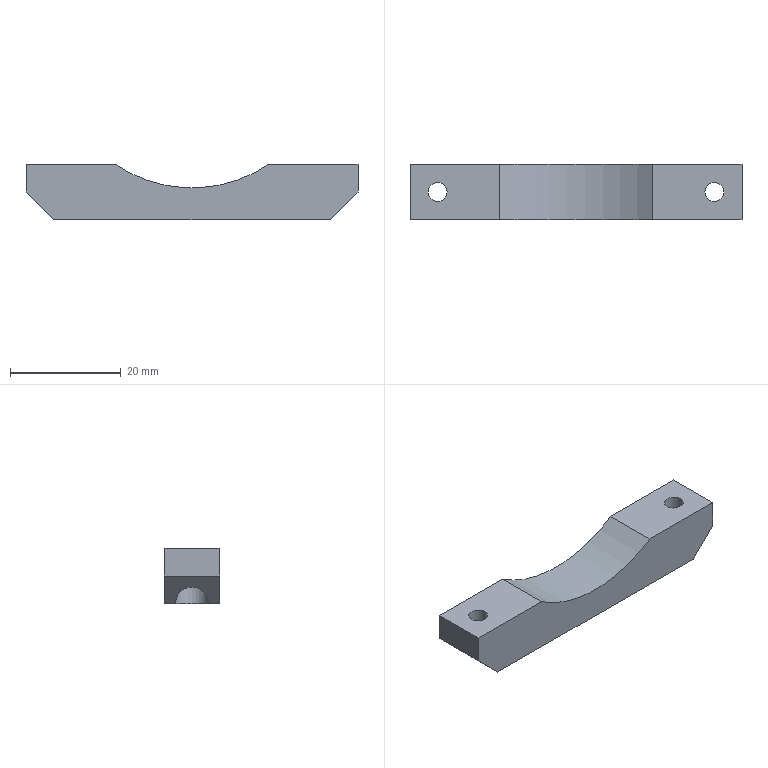Part | STEP file | SynoNew-0304-067 | 1 solid | 16 faces | box 60 x 10 x 10 mm | volume 4574 mm3 | plane 11 | cylinder 5 | commonest cylinder face diameters 3.4 x2 6 x2 49.5 x1
STEP:
#1=CARTESIAN_POINT('',(0.,10.,-5.));
#2=VERTEX_POINT('',#1);
#3=CARTESIAN_POINT('',(0.,10.,0.));
#4=VERTEX_POINT('',#3);
#5=CARTESIAN_POINT('',(0.,10.,-5.));
#6=DIRECTION('',(0.,0.,1.));
#7=VECTOR('',#6,5.);
#8=LINE('',#5,#7);
#9=EDGE_CURVE('',#2,#4,#8,.T.);
#10=ORIENTED_EDGE('',*,*,#9,.F.);
#11=CARTESIAN_POINT('',(0.,0.,-5.));
#12=VERTEX_POINT('',#11);
#13=CARTESIAN_POINT('',(0.,10.,-5.));
#14=DIRECTION('',(0.,-1.,0.));
#15=VECTOR('',#14,10.);
#16=LINE('',#13,#15);
#17=EDGE_CURVE('',#2,#12,#16,.T.);
#18=ORIENTED_EDGE('',*,*,#17,.T.);
#19=CARTESIAN_POINT('',(0.,0.,0.));
#20=VERTEX_POINT('',#19);
#21=CARTESIAN_POINT('',(0.,0.,-5.));
#22=DIRECTION('',(0.,0.,1.));
#23=VECTOR('',#22,5.);
#24=LINE('',#21,#23);
#25=EDGE_CURVE('',#12,#20,#24,.T.);
#26=ORIENTED_EDGE('',*,*,#25,.T.);
#27=CARTESIAN_POINT('',(0.,10.,0.));
#28=DIRECTION('',(0.,-1.,0.));
#29=VECTOR('',#28,10.);
#30=LINE('',#27,#29);
#31=EDGE_CURVE('',#4,#20,#30,.T.);
#32=ORIENTED_EDGE('',*,*,#31,.F.);
#33=EDGE_LOOP('',(#10,#18,#26,#32));
#34=FACE_OUTER_BOUND('',#33,.T.);
#35=CARTESIAN_POINT('',(0.,10.,0.));
#36=DIRECTION('',(1.,0.,0.));
#37=DIRECTION('',(0.,0.,-1.));
#38=AXIS2_PLACEMENT_3D('',#35,#36,#37);
#39=PLANE('',#38);
#40=ADVANCED_FACE('',(#34),#39,.F.);
#41=CARTESIAN_POINT('',(16.132,0.,0.));
#42=VERTEX_POINT('',#41);
#43=CARTESIAN_POINT('',(0.,0.,0.));
#44=DIRECTION('',(1.,0.,0.));
#45=VECTOR('',#44,16.132);
#46=LINE('',#43,#45);
#47=EDGE_CURVE('',#20,#42,#46,.T.);
#48=ORIENTED_EDGE('',*,*,#47,.T.);
#49=CARTESIAN_POINT('',(16.132,10.,0.));
#50=VERTEX_POINT('',#49);
#51=CARTESIAN_POINT('',(16.132,10.,0.));
#52=DIRECTION('',(0.,-1.,0.));
#53=VECTOR('',#52,10.);
#54=LINE('',#51,#53);
#55=EDGE_CURVE('',#50,#42,#54,.T.);
#56=ORIENTED_EDGE('',*,*,#55,.F.);
#57=CARTESIAN_POINT('',(0.,10.,0.));
#58=DIRECTION('',(1.,0.,0.));
#59=VECTOR('',#58,16.132);
#60=LINE('',#57,#59);
#61=EDGE_CURVE('',#4,#50,#60,.T.);
#62=ORIENTED_EDGE('',*,*,#61,.F.);
#63=ORIENTED_EDGE('',*,*,#31,.T.);
#64=EDGE_LOOP('',(#48,#56,#62,#63));
#65=FACE_OUTER_BOUND('',#64,.T.);
#66=CARTESIAN_POINT('',(3.3,5.,0.));
#67=VERTEX_POINT('',#66);
#68=CARTESIAN_POINT('',(6.7,5.,0.));
#69=VERTEX_POINT('',#68);
#70=CARTESIAN_POINT('',(5.,5.,0.));
#71=DIRECTION('',(0.,0.,-1.));
#72=DIRECTION('',(-1.,0.,0.));
#73=AXIS2_PLACEMENT_3D('',#70,#71,#72);
#74=CIRCLE('',#73,1.7);
#75=EDGE_CURVE('',#67,#69,#74,.T.);
#76=ORIENTED_EDGE('',*,*,#75,.T.);
#77=CARTESIAN_POINT('',(5.,5.,0.));
#78=DIRECTION('',(0.,0.,-1.));
#79=DIRECTION('',(-1.,0.,0.));
#80=AXIS2_PLACEMENT_3D('',#77,#78,#79);
#81=CIRCLE('',#80,1.7);
#82=EDGE_CURVE('',#69,#67,#81,.T.);
#83=ORIENTED_EDGE('',*,*,#82,.T.);
#84=EDGE_LOOP('',(#76,#83));
#85=FACE_BOUND('',#84,.T.);
#86=CARTESIAN_POINT('',(0.,10.,0.));
#87=DIRECTION('',(0.,0.,-1.));
#88=DIRECTION('',(-1.,0.,0.));
#89=AXIS2_PLACEMENT_3D('',#86,#87,#88);
#90=PLANE('',#89);
#91=ADVANCED_FACE('',(#65,#85),#90,.F.);
#92=CARTESIAN_POINT('',(43.868,0.,0.));
#93=VERTEX_POINT('',#92);
#94=CARTESIAN_POINT('',(30.,0.,20.5));
#95=DIRECTION('',(0.,-1.,0.));
#96=DIRECTION('',(0.,0.,1.));
#97=AXIS2_PLACEMENT_3D('',#94,#95,#96);
#98=CIRCLE('',#97,24.75);
#99=EDGE_CURVE('',#42,#93,#98,.T.);
#100=ORIENTED_EDGE('',*,*,#99,.T.);
#101=CARTESIAN_POINT('',(43.868,10.,0.));
#102=VERTEX_POINT('',#101);
#103=CARTESIAN_POINT('',(43.868,10.,0.));
#104=DIRECTION('',(0.,-1.,0.));
#105=VECTOR('',#104,10.);
#106=LINE('',#103,#105);
#107=EDGE_CURVE('',#102,#93,#106,.T.);
#108=ORIENTED_EDGE('',*,*,#107,.F.);
#109=CARTESIAN_POINT('',(30.,10.,20.5));
#110=DIRECTION('',(0.,-1.,0.));
#111=DIRECTION('',(0.,0.,1.));
#112=AXIS2_PLACEMENT_3D('',#109,#110,#111);
#113=CIRCLE('',#112,24.75);
#114=EDGE_CURVE('',#50,#102,#113,.T.);
#115=ORIENTED_EDGE('',*,*,#114,.F.);
#116=ORIENTED_EDGE('',*,*,#55,.T.);
#117=EDGE_LOOP('',(#100,#108,#115,#116));
#118=FACE_OUTER_BOUND('',#117,.T.);
#119=CARTESIAN_POINT('',(30.,10.,20.5));
#120=DIRECTION('',(0.,-1.,0.));
#121=DIRECTION('',(0.,0.,-1.));
#122=AXIS2_PLACEMENT_3D('',#119,#120,#121);
#123=CYLINDRICAL_SURFACE('',#122,24.75);
#124=ADVANCED_FACE('',(#118),#123,.F.);
#125=CARTESIAN_POINT('',(60.,0.,0.));
#126=VERTEX_POINT('',#125);
#127=CARTESIAN_POINT('',(43.868,0.,0.));
#128=DIRECTION('',(1.,0.,0.));
#129=VECTOR('',#128,16.132);
#130=LINE('',#127,#129);
#131=EDGE_CURVE('',#93,#126,#130,.T.);
#132=ORIENTED_EDGE('',*,*,#131,.T.);
#133=CARTESIAN_POINT('',(60.,10.,0.));
#134=VERTEX_POINT('',#133);
#135=CARTESIAN_POINT('',(60.,10.,0.));
#136=DIRECTION('',(0.,-1.,0.));
#137=VECTOR('',#136,10.);
#138=LINE('',#135,#137);
#139=EDGE_CURVE('',#134,#126,#138,.T.);
#140=ORIENTED_EDGE('',*,*,#139,.F.);
#141=CARTESIAN_POINT('',(43.868,10.,0.));
#142=DIRECTION('',(1.,0.,0.));
#143=VECTOR('',#142,16.132);
#144=LINE('',#141,#143);
#145=EDGE_CURVE('',#102,#134,#144,.T.);
#146=ORIENTED_EDGE('',*,*,#145,.F.);
#147=ORIENTED_EDGE('',*,*,#107,.T.);
#148=EDGE_LOOP('',(#132,#140,#146,#147));
#149=FACE_OUTER_BOUND('',#148,.T.);
#150=CARTESIAN_POINT('',(53.3,5.,0.));
#151=VERTEX_POINT('',#150);
#152=CARTESIAN_POINT('',(56.7,5.,0.));
#153=VERTEX_POINT('',#152);
#154=CARTESIAN_POINT('',(55.,5.,0.));
#155=DIRECTION('',(0.,0.,-1.));
#156=DIRECTION('',(-1.,0.,0.));
#157=AXIS2_PLACEMENT_3D('',#154,#155,#156);
#158=CIRCLE('',#157,1.7);
#159=EDGE_CURVE('',#151,#153,#158,.T.);
#160=ORIENTED_EDGE('',*,*,#159,.T.);
#161=CARTESIAN_POINT('',(55.,5.,0.));
#162=DIRECTION('',(0.,0.,-1.));
#163=DIRECTION('',(-1.,0.,0.));
#164=AXIS2_PLACEMENT_3D('',#161,#162,#163);
#165=CIRCLE('',#164,1.7);
#166=EDGE_CURVE('',#153,#151,#165,.T.);
#167=ORIENTED_EDGE('',*,*,#166,.T.);
#168=EDGE_LOOP('',(#160,#167));
#169=FACE_BOUND('',#168,.T.);
#170=CARTESIAN_POINT('',(43.868,10.,0.));
#171=DIRECTION('',(0.,0.,-1.));
#172=DIRECTION('',(-1.,0.,0.));
#173=AXIS2_PLACEMENT_3D('',#170,#171,#172);
#174=PLANE('',#173);
#175=ADVANCED_FACE('',(#149,#169),#174,.F.);
#176=CARTESIAN_POINT('',(60.,0.,-5.));
#177=VERTEX_POINT('',#176);
#178=CARTESIAN_POINT('',(60.,0.,0.));
#179=DIRECTION('',(0.,0.,-1.));
#180=VECTOR('',#179,5.);
#181=LINE('',#178,#180);
#182=EDGE_CURVE('',#126,#177,#181,.T.);
#183=ORIENTED_EDGE('',*,*,#182,.T.);
#184=CARTESIAN_POINT('',(60.,10.,-5.));
#185=VERTEX_POINT('',#184);
#186=CARTESIAN_POINT('',(60.,0.,-5.));
#187=DIRECTION('',(0.,1.,0.));
#188=VECTOR('',#187,10.);
#189=LINE('',#186,#188);
#190=EDGE_CURVE('',#177,#185,#189,.T.);
#191=ORIENTED_EDGE('',*,*,#190,.T.);
#192=CARTESIAN_POINT('',(60.,10.,0.));
#193=DIRECTION('',(0.,0.,-1.));
#194=VECTOR('',#193,5.);
#195=LINE('',#192,#194);
#196=EDGE_CURVE('',#134,#185,#195,.T.);
#197=ORIENTED_EDGE('',*,*,#196,.F.);
#198=ORIENTED_EDGE('',*,*,#139,.T.);
#199=EDGE_LOOP('',(#183,#191,#197,#198));
#200=FACE_OUTER_BOUND('',#199,.T.);
#201=CARTESIAN_POINT('',(60.,10.,0.));
#202=DIRECTION('',(-1.,0.,0.));
#203=DIRECTION('',(0.,0.,1.));
#204=AXIS2_PLACEMENT_3D('',#201,#202,#203);
#205=PLANE('',#204);
#206=ADVANCED_FACE('',(#200),#205,.F.);
#207=CARTESIAN_POINT('',(55.,10.,-10.));
#208=VERTEX_POINT('',#207);
#209=CARTESIAN_POINT('',(55.,8.,-10.));
#210=VERTEX_POINT('',#209);
#211=CARTESIAN_POINT('',(55.,10.,-10.));
#212=DIRECTION('',(0.,-1.,0.));
#213=VECTOR('',#212,2.);
#214=LINE('',#211,#213);
#215=EDGE_CURVE('',#208,#210,#214,.T.);
#216=ORIENTED_EDGE('',*,*,#215,.T.);
#217=CARTESIAN_POINT('',(55.,2.,-10.));
#218=VERTEX_POINT('',#217);
#219=CARTESIAN_POINT('',(55.,5.,-10.));
#220=DIRECTION('',(0.,0.,-1.));
#221=DIRECTION('',(-1.,0.,0.));
#222=AXIS2_PLACEMENT_3D('',#219,#220,#221);
#223=CIRCLE('',#222,3.);
#224=EDGE_CURVE('',#218,#210,#223,.T.);
#225=ORIENTED_EDGE('',*,*,#224,.F.);
#226=CARTESIAN_POINT('',(55.,0.,-10.));
#227=VERTEX_POINT('',#226);
#228=CARTESIAN_POINT('',(55.,2.,-10.));
#229=DIRECTION('',(0.,-1.,0.));
#230=VECTOR('',#229,2.);
#231=LINE('',#228,#230);
#232=EDGE_CURVE('',#218,#227,#231,.T.);
#233=ORIENTED_EDGE('',*,*,#232,.T.);
#234=CARTESIAN_POINT('',(5.,0.,-10.));
#235=VERTEX_POINT('',#234);
#236=CARTESIAN_POINT('',(55.,0.,-10.));
#237=DIRECTION('',(-1.,0.,0.));
#238=VECTOR('',#237,50.);
#239=LINE('',#236,#238);
#240=EDGE_CURVE('',#227,#235,#239,.T.);
#241=ORIENTED_EDGE('',*,*,#240,.T.);
#242=CARTESIAN_POINT('',(5.,2.,-10.));
#243=VERTEX_POINT('',#242);
#244=CARTESIAN_POINT('',(5.,0.,-10.));
#245=DIRECTION('',(0.,1.,0.));
#246=VECTOR('',#245,2.);
#247=LINE('',#244,#246);
#248=EDGE_CURVE('',#235,#243,#247,.T.);
#249=ORIENTED_EDGE('',*,*,#248,.T.);
#250=CARTESIAN_POINT('',(8.,5.,-10.));
#251=VERTEX_POINT('',#250);
#252=CARTESIAN_POINT('',(5.,5.,-10.));
#253=DIRECTION('',(0.,0.,-1.));
#254=DIRECTION('',(-1.,0.,0.));
#255=AXIS2_PLACEMENT_3D('',#252,#253,#254);
#256=CIRCLE('',#255,3.);
#257=EDGE_CURVE('',#251,#243,#256,.T.);
#258=ORIENTED_EDGE('',*,*,#257,.F.);
#259=CARTESIAN_POINT('',(5.,8.,-10.));
#260=VERTEX_POINT('',#259);
#261=CARTESIAN_POINT('',(5.,5.,-10.));
#262=DIRECTION('',(0.,0.,-1.));
#263=DIRECTION('',(-1.,0.,0.));
#264=AXIS2_PLACEMENT_3D('',#261,#262,#263);
#265=CIRCLE('',#264,3.);
#266=EDGE_CURVE('',#260,#251,#265,.T.);
#267=ORIENTED_EDGE('',*,*,#266,.F.);
#268=CARTESIAN_POINT('',(5.,10.,-10.));
#269=VERTEX_POINT('',#268);
#270=CARTESIAN_POINT('',(5.,8.,-10.));
#271=DIRECTION('',(0.,1.,0.));
#272=VECTOR('',#271,2.);
#273=LINE('',#270,#272);
#274=EDGE_CURVE('',#260,#269,#273,.T.);
#275=ORIENTED_EDGE('',*,*,#274,.T.);
#276=CARTESIAN_POINT('',(55.,10.,-10.));
#277=DIRECTION('',(-1.,0.,0.));
#278=VECTOR('',#277,50.);
#279=LINE('',#276,#278);
#280=EDGE_CURVE('',#208,#269,#279,.T.);
#281=ORIENTED_EDGE('',*,*,#280,.F.);
#282=EDGE_LOOP('',(#216,#225,#233,#241,#249,#258,#267,#275,#281));
#283=FACE_OUTER_BOUND('',#282,.T.);
#284=CARTESIAN_POINT('',(0.,10.,-10.));
#285=DIRECTION('',(0.,0.,1.));
#286=DIRECTION('',(1.,0.,0.));
#287=AXIS2_PLACEMENT_3D('',#284,#285,#286);
#288=PLANE('',#287);
#289=ADVANCED_FACE('',(#283),#288,.F.);
#290=ORIENTED_EDGE('',*,*,#196,.T.);
#291=CARTESIAN_POINT('',(55.,10.,-10.));
#292=DIRECTION('',(0.7071,0.,0.7071));
#293=VECTOR('',#292,7.071);
#294=LINE('',#291,#293);
#295=EDGE_CURVE('',#185,#208,#294,.F.);
#296=ORIENTED_EDGE('',*,*,#295,.T.);
#297=ORIENTED_EDGE('',*,*,#280,.T.);
#298=CARTESIAN_POINT('',(0.,10.,-5.));
#299=DIRECTION('',(0.7071,0.,-0.7071));
#300=VECTOR('',#299,7.071);
#301=LINE('',#298,#300);
#302=EDGE_CURVE('',#269,#2,#301,.F.);
#303=ORIENTED_EDGE('',*,*,#302,.T.);
#304=ORIENTED_EDGE('',*,*,#9,.T.);
#305=ORIENTED_EDGE('',*,*,#61,.T.);
#306=ORIENTED_EDGE('',*,*,#114,.T.);
#307=ORIENTED_EDGE('',*,*,#145,.T.);
#308=EDGE_LOOP('',(#290,#296,#297,#303,#304,#305,#306,#307));
#309=FACE_OUTER_BOUND('',#308,.T.);
#310=CARTESIAN_POINT('',(30.,10.,20.5));
#311=DIRECTION('',(0.,1.,0.));
#312=DIRECTION('',(0.,0.,1.));
#313=AXIS2_PLACEMENT_3D('',#310,#311,#312);
#314=PLANE('',#313);
#315=ADVANCED_FACE('',(#309),#314,.T.);
#316=ORIENTED_EDGE('',*,*,#240,.F.);
#317=CARTESIAN_POINT('',(60.,0.,-5.));
#318=DIRECTION('',(-0.7071,0.,-0.7071));
#319=VECTOR('',#318,7.071);
#320=LINE('',#317,#319);
#321=EDGE_CURVE('',#227,#177,#320,.F.);
#322=ORIENTED_EDGE('',*,*,#321,.T.);
#323=ORIENTED_EDGE('',*,*,#182,.F.);
#324=ORIENTED_EDGE('',*,*,#131,.F.);
#325=ORIENTED_EDGE('',*,*,#99,.F.);
#326=ORIENTED_EDGE('',*,*,#47,.F.);
#327=ORIENTED_EDGE('',*,*,#25,.F.);
#328=CARTESIAN_POINT('',(5.,0.,-10.));
#329=DIRECTION('',(-0.7071,0.,0.7071));
#330=VECTOR('',#329,7.071);
#331=LINE('',#328,#330);
#332=EDGE_CURVE('',#12,#235,#331,.F.);
#333=ORIENTED_EDGE('',*,*,#332,.T.);
#334=EDGE_LOOP('',(#316,#322,#323,#324,#325,#326,#327,#333));
#335=FACE_OUTER_BOUND('',#334,.T.);
#336=CARTESIAN_POINT('',(30.,0.,20.5));
#337=DIRECTION('',(0.,1.,0.));
#338=DIRECTION('',(0.,0.,1.));
#339=AXIS2_PLACEMENT_3D('',#336,#337,#338);
#340=PLANE('',#339);
#341=ADVANCED_FACE('',(#335),#340,.F.);
#342=CARTESIAN_POINT('',(58.,5.,-7.));
#343=VERTEX_POINT('',#342);
#344=CARTESIAN_POINT('',(55.,5.,-10.));
#345=DIRECTION('',(-0.7071,0.,0.7071));
#346=DIRECTION('',(-0.7071,0.,-0.7071));
#347=AXIS2_PLACEMENT_3D('',#344,#345,#346);
#348=ELLIPSE('',#347,4.243,3.);
#349=EDGE_CURVE('',#210,#343,#348,.F.);
#350=ORIENTED_EDGE('',*,*,#349,.F.);
#351=ORIENTED_EDGE('',*,*,#215,.F.);
#352=ORIENTED_EDGE('',*,*,#295,.F.);
#353=ORIENTED_EDGE('',*,*,#190,.F.);
#354=ORIENTED_EDGE('',*,*,#321,.F.);
#355=ORIENTED_EDGE('',*,*,#232,.F.);
#356=CARTESIAN_POINT('',(55.,5.,-10.));
#357=DIRECTION('',(-0.7071,0.,0.7071));
#358=DIRECTION('',(-0.7071,0.,-0.7071));
#359=AXIS2_PLACEMENT_3D('',#356,#357,#358);
#360=ELLIPSE('',#359,4.243,3.);
#361=EDGE_CURVE('',#343,#218,#360,.F.);
#362=ORIENTED_EDGE('',*,*,#361,.F.);
#363=EDGE_LOOP('',(#350,#351,#352,#353,#354,#355,#362));
#364=FACE_OUTER_BOUND('',#363,.T.);
#365=CARTESIAN_POINT('',(55.,10.,-10.));
#366=DIRECTION('',(-0.7071,0.,0.7071));
#367=DIRECTION('',(0.7071,0.,0.7071));
#368=AXIS2_PLACEMENT_3D('',#365,#366,#367);
#369=PLANE('',#368);
#370=ADVANCED_FACE('',(#364),#369,.F.);
#371=CARTESIAN_POINT('',(5.,5.,-10.));
#372=DIRECTION('',(0.7071,0.,0.7071));
#373=DIRECTION('',(0.7071,0.,-0.7071));
#374=AXIS2_PLACEMENT_3D('',#371,#372,#373);
#375=ELLIPSE('',#374,4.243,3.);
#376=EDGE_CURVE('',#243,#260,#375,.F.);
#377=ORIENTED_EDGE('',*,*,#376,.F.);
#378=ORIENTED_EDGE('',*,*,#248,.F.);
#379=ORIENTED_EDGE('',*,*,#332,.F.);
#380=ORIENTED_EDGE('',*,*,#17,.F.);
#381=ORIENTED_EDGE('',*,*,#302,.F.);
#382=ORIENTED_EDGE('',*,*,#274,.F.);
#383=EDGE_LOOP('',(#377,#378,#379,#380,#381,#382));
#384=FACE_OUTER_BOUND('',#383,.T.);
#385=CARTESIAN_POINT('',(0.,10.,-5.));
#386=DIRECTION('',(0.7071,0.,0.7071));
#387=DIRECTION('',(0.7071,0.,-0.7071));
#388=AXIS2_PLACEMENT_3D('',#385,#386,#387);
#389=PLANE('',#388);
#390=ADVANCED_FACE('',(#384),#389,.F.);
#391=ORIENTED_EDGE('',*,*,#75,.F.);
#392=ORIENTED_EDGE('',*,*,#82,.F.);
#393=CARTESIAN_POINT('',(6.7,5.,-4.));
#394=VERTEX_POINT('',#393);
#395=CARTESIAN_POINT('',(6.7,5.,-10.));
#396=DIRECTION('',(0.,0.,-1.));
#397=VECTOR('',#396,1.7);
#398=LINE('',#395,#397);
#399=EDGE_CURVE('',#69,#394,#398,.T.);
#400=ORIENTED_EDGE('',*,*,#399,.T.);
#401=CARTESIAN_POINT('',(3.3,5.,-4.));
#402=VERTEX_POINT('',#401);
#403=CARTESIAN_POINT('',(5.,5.,-4.));
#404=DIRECTION('',(0.,0.,-1.));
#405=DIRECTION('',(-1.,0.,0.));
#406=AXIS2_PLACEMENT_3D('',#403,#404,#405);
#407=CIRCLE('',#406,1.7);
#408=EDGE_CURVE('',#394,#402,#407,.T.);
#409=ORIENTED_EDGE('',*,*,#408,.T.);
#410=CARTESIAN_POINT('',(5.,5.,-4.));
#411=DIRECTION('',(0.,0.,-1.));
#412=DIRECTION('',(-1.,0.,0.));
#413=AXIS2_PLACEMENT_3D('',#410,#411,#412);
#414=CIRCLE('',#413,1.7);
#415=EDGE_CURVE('',#402,#394,#414,.T.);
#416=ORIENTED_EDGE('',*,*,#415,.T.);
#417=ORIENTED_EDGE('',*,*,#399,.F.);
#418=EDGE_LOOP('',(#391,#392,#400,#409,#416,#417));
#419=FACE_OUTER_BOUND('',#418,.T.);
#420=CARTESIAN_POINT('',(5.,5.,-10.));
#421=DIRECTION('',(0.,0.,-1.));
#422=DIRECTION('',(-1.,0.,0.));
#423=AXIS2_PLACEMENT_3D('',#420,#421,#422);
#424=CYLINDRICAL_SURFACE('',#423,1.7);
#425=ADVANCED_FACE('',(#419),#424,.F.);
#426=CARTESIAN_POINT('',(2.,5.,-4.));
#427=VERTEX_POINT('',#426);
#428=CARTESIAN_POINT('',(8.,5.,-4.));
#429=VERTEX_POINT('',#428);
#430=CARTESIAN_POINT('',(5.,5.,-4.));
#431=DIRECTION('',(0.,0.,-1.));
#432=DIRECTION('',(-1.,0.,0.));
#433=AXIS2_PLACEMENT_3D('',#430,#431,#432);
#434=CIRCLE('',#433,3.);
#435=EDGE_CURVE('',#427,#429,#434,.T.);
#436=ORIENTED_EDGE('',*,*,#435,.T.);
#437=CARTESIAN_POINT('',(5.,5.,-4.));
#438=DIRECTION('',(0.,0.,-1.));
#439=DIRECTION('',(-1.,0.,0.));
#440=AXIS2_PLACEMENT_3D('',#437,#438,#439);
#441=CIRCLE('',#440,3.);
#442=EDGE_CURVE('',#429,#427,#441,.T.);
#443=ORIENTED_EDGE('',*,*,#442,.T.);
#444=EDGE_LOOP('',(#436,#443));
#445=FACE_OUTER_BOUND('',#444,.T.);
#446=ORIENTED_EDGE('',*,*,#415,.F.);
#447=ORIENTED_EDGE('',*,*,#408,.F.);
#448=EDGE_LOOP('',(#446,#447));
#449=FACE_BOUND('',#448,.T.);
#450=CARTESIAN_POINT('',(6.7,5.,-4.));
#451=DIRECTION('',(0.,0.,1.));
#452=DIRECTION('',(1.,0.,0.));
#453=AXIS2_PLACEMENT_3D('',#450,#451,#452);
#454=PLANE('',#453);
#455=ADVANCED_FACE('',(#445,#449),#454,.F.);
#456=ORIENTED_EDGE('',*,*,#435,.F.);
#457=ORIENTED_EDGE('',*,*,#442,.F.);
#458=CARTESIAN_POINT('',(8.,5.,-10.));
#459=DIRECTION('',(0.,0.,-1.));
#460=VECTOR('',#459,3.);
#461=LINE('',#458,#460);
#462=EDGE_CURVE('',#429,#251,#461,.T.);
#463=ORIENTED_EDGE('',*,*,#462,.T.);
#464=ORIENTED_EDGE('',*,*,#257,.T.);
#465=ORIENTED_EDGE('',*,*,#376,.T.);
#466=ORIENTED_EDGE('',*,*,#266,.T.);
#467=ORIENTED_EDGE('',*,*,#462,.F.);
#468=EDGE_LOOP('',(#456,#457,#463,#464,#465,#466,#467));
#469=FACE_OUTER_BOUND('',#468,.T.);
#470=CARTESIAN_POINT('',(5.,5.,-10.));
#471=DIRECTION('',(0.,0.,-1.));
#472=DIRECTION('',(-1.,0.,0.));
#473=AXIS2_PLACEMENT_3D('',#470,#471,#472);
#474=CYLINDRICAL_SURFACE('',#473,3.);
#475=ADVANCED_FACE('',(#469),#474,.F.);
#476=ORIENTED_EDGE('',*,*,#159,.F.);
#477=ORIENTED_EDGE('',*,*,#166,.F.);
#478=CARTESIAN_POINT('',(56.7,5.,-4.));
#479=VERTEX_POINT('',#478);
#480=CARTESIAN_POINT('',(56.7,5.,-10.));
#481=DIRECTION('',(0.,0.,-1.));
#482=VECTOR('',#481,1.7);
#483=LINE('',#480,#482);
#484=EDGE_CURVE('',#153,#479,#483,.T.);
#485=ORIENTED_EDGE('',*,*,#484,.T.);
#486=CARTESIAN_POINT('',(53.3,5.,-4.));
#487=VERTEX_POINT('',#486);
#488=CARTESIAN_POINT('',(55.,5.,-4.));
#489=DIRECTION('',(0.,0.,-1.));
#490=DIRECTION('',(-1.,0.,0.));
#491=AXIS2_PLACEMENT_3D('',#488,#489,#490);
#492=CIRCLE('',#491,1.7);
#493=EDGE_CURVE('',#479,#487,#492,.T.);
#494=ORIENTED_EDGE('',*,*,#493,.T.);
#495=CARTESIAN_POINT('',(55.,5.,-4.));
#496=DIRECTION('',(0.,0.,-1.));
#497=DIRECTION('',(-1.,0.,0.));
#498=AXIS2_PLACEMENT_3D('',#495,#496,#497);
#499=CIRCLE('',#498,1.7);
#500=EDGE_CURVE('',#487,#479,#499,.T.);
#501=ORIENTED_EDGE('',*,*,#500,.T.);
#502=ORIENTED_EDGE('',*,*,#484,.F.);
#503=EDGE_LOOP('',(#476,#477,#485,#494,#501,#502));
#504=FACE_OUTER_BOUND('',#503,.T.);
#505=CARTESIAN_POINT('',(55.,5.,-10.));
#506=DIRECTION('',(0.,0.,-1.));
#507=DIRECTION('',(-1.,0.,0.));
#508=AXIS2_PLACEMENT_3D('',#505,#506,#507);
#509=CYLINDRICAL_SURFACE('',#508,1.7);
#510=ADVANCED_FACE('',(#504),#509,.F.);
#511=CARTESIAN_POINT('',(52.,5.,-4.));
#512=VERTEX_POINT('',#511);
#513=CARTESIAN_POINT('',(58.,5.,-4.));
#514=VERTEX_POINT('',#513);
#515=CARTESIAN_POINT('',(55.,5.,-4.));
#516=DIRECTION('',(0.,0.,-1.));
#517=DIRECTION('',(-1.,0.,0.));
#518=AXIS2_PLACEMENT_3D('',#515,#516,#517);
#519=CIRCLE('',#518,3.);
#520=EDGE_CURVE('',#512,#514,#519,.T.);
#521=ORIENTED_EDGE('',*,*,#520,.T.);
#522=CARTESIAN_POINT('',(55.,5.,-4.));
#523=DIRECTION('',(0.,0.,-1.));
#524=DIRECTION('',(-1.,0.,0.));
#525=AXIS2_PLACEMENT_3D('',#522,#523,#524);
#526=CIRCLE('',#525,3.);
#527=EDGE_CURVE('',#514,#512,#526,.T.);
#528=ORIENTED_EDGE('',*,*,#527,.T.);
#529=EDGE_LOOP('',(#521,#528));
#530=FACE_OUTER_BOUND('',#529,.T.);
#531=ORIENTED_EDGE('',*,*,#500,.F.);
#532=ORIENTED_EDGE('',*,*,#493,.F.);
#533=EDGE_LOOP('',(#531,#532));
#534=FACE_BOUND('',#533,.T.);
#535=CARTESIAN_POINT('',(56.7,5.,-4.));
#536=DIRECTION('',(0.,0.,1.));
#537=DIRECTION('',(1.,0.,0.));
#538=AXIS2_PLACEMENT_3D('',#535,#536,#537);
#539=PLANE('',#538);
#540=ADVANCED_FACE('',(#530,#534),#539,.F.);
#541=ORIENTED_EDGE('',*,*,#520,.F.);
#542=ORIENTED_EDGE('',*,*,#527,.F.);
#543=CARTESIAN_POINT('',(58.,5.,-10.));
#544=DIRECTION('',(0.,0.,-1.));
#545=VECTOR('',#544,3.);
#546=LINE('',#543,#545);
#547=EDGE_CURVE('',#514,#343,#546,.T.);
#548=ORIENTED_EDGE('',*,*,#547,.T.);
#549=ORIENTED_EDGE('',*,*,#361,.T.);
#550=ORIENTED_EDGE('',*,*,#224,.T.);
#551=ORIENTED_EDGE('',*,*,#349,.T.);
#552=ORIENTED_EDGE('',*,*,#547,.F.);
#553=EDGE_LOOP('',(#541,#542,#548,#549,#550,#551,#552));
#554=FACE_OUTER_BOUND('',#553,.T.);
#555=CARTESIAN_POINT('',(55.,5.,-10.));
#556=DIRECTION('',(0.,0.,-1.));
#557=DIRECTION('',(-1.,0.,0.));
#558=AXIS2_PLACEMENT_3D('',#555,#556,#557);
#559=CYLINDRICAL_SURFACE('',#558,3.);
#560=ADVANCED_FACE('',(#554),#559,.F.);
#561=CLOSED_SHELL('',(#40,#91,#124,#175,#206,#289,#315,#341,#370,#390,#425,#455,#475,#510,#540,#560));
#562=MANIFOLD_SOLID_BREP('',#561);
#563=(LENGTH_UNIT()NAMED_UNIT(*)SI_UNIT(.MILLI.,.METRE.));
#564=UNCERTAINTY_MEASURE_WITH_UNIT(LENGTH_MEASURE(0.01),#563,'','');
#565=(NAMED_UNIT(*)PLANE_ANGLE_UNIT()SI_UNIT($,.RADIAN.));
#566=(NAMED_UNIT(*)SI_UNIT($,.STERADIAN.)SOLID_ANGLE_UNIT());
#567=(GEOMETRIC_REPRESENTATION_CONTEXT(3)GLOBAL_UNCERTAINTY_ASSIGNED_CONTEXT((#564))GLOBAL_UNIT_ASSIGNED_CONTEXT((#563,#565,#566))REPRESENTATION_CONTEXT('',''));
#568=ADVANCED_BREP_SHAPE_REPRESENTATION('',(#562),#567);